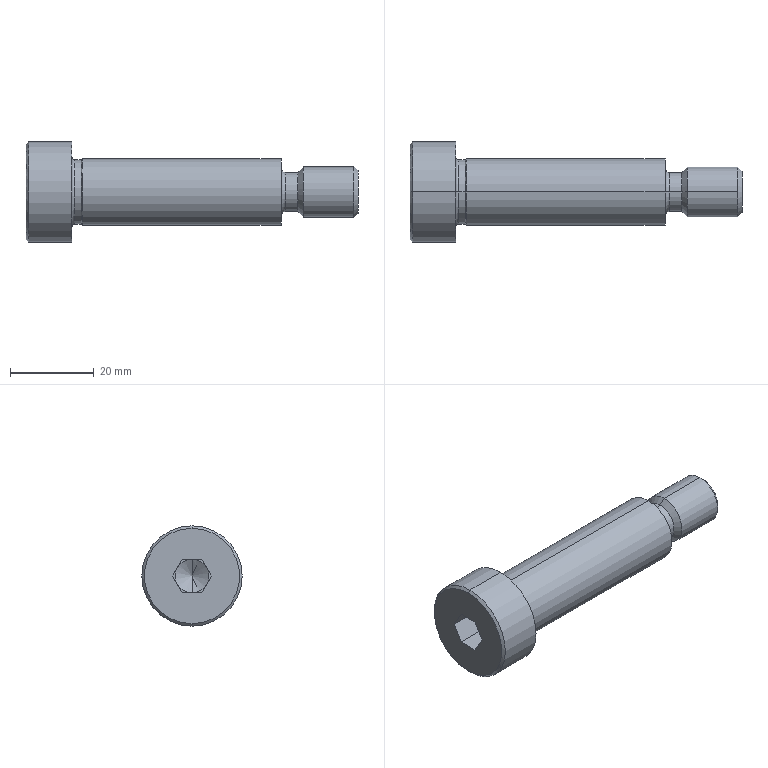Part | STEP file | socket head shoulder screw2_am_B18.3.3M - 16 x 50 SHSS --N | 1 solid | 40 faces | box 79.4 x 24 x 24 mm | volume 16413 mm3 | plane 16 | cone 10 | cylinder 10 | torus 4 | commonest cylinder face diameters 9.35 x2 12 x2 15.42 x2 15.984 x2 24 x2